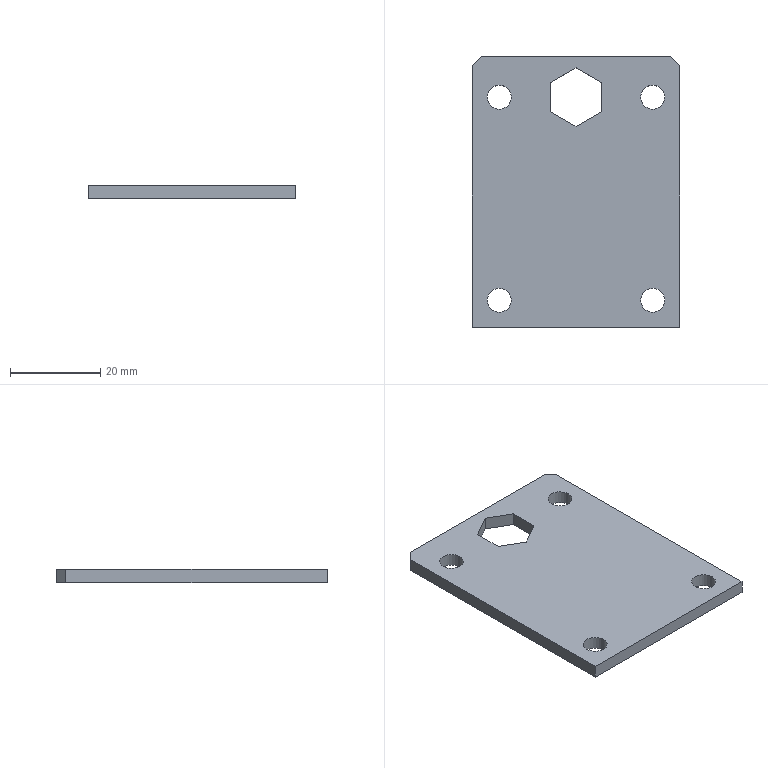Part | STEP file | Z-081D | 1 solid | 18 faces | box 46 x 60 x 2.9 mm | volume 7421 mm3 | plane 14 | cylinder 4 | commonest cylinder face diameters 5.3 x4
STEP:
#1=CARTESIAN_POINT('',(0.,0.,0.));
#2=DIRECTION('',(0.,0.,1.));
#3=DIRECTION('',(1.,0.,0.));
#4=AXIS2_PLACEMENT_3D('',#1,#2,#3);
#5=CARTESIAN_POINT('',(17.4,54.233,2.9));
#6=VERTEX_POINT('',#5);
#7=CARTESIAN_POINT('',(23.,57.466,2.9));
#8=VERTEX_POINT('',#7);
#9=CARTESIAN_POINT('',(14.253,52.416,2.9));
#10=DIRECTION('',(0.866,0.5,0.));
#11=VECTOR('',#10,1.);
#12=LINE('',#9,#11);
#13=CARTESIAN_POINT('',(17.4,54.233,2.9));
#14=DIRECTION('',(-0.5,0.866,0.));
#15=DIRECTION('',(0.866,0.5,0.));
#16=AXIS2_PLACEMENT_3D('',#13,#14,#15);
#17=PLANE('',#16);
#18=CARTESIAN_POINT('',(-3.633,0.));
#19=DIRECTION('',(1.,0.));
#20=VECTOR('',#19,1.);
#21=LINE('',#18,#20);
#22=(GEOMETRIC_REPRESENTATION_CONTEXT(2)PARAMETRIC_REPRESENTATION_CONTEXT()REPRESENTATION_CONTEXT('',''));
#23=DEFINITIONAL_REPRESENTATION('',(#21),#22);
#24=PCURVE('',#17,#23);
#25=CARTESIAN_POINT('',(23.,30.,2.9));
#26=DIRECTION('',(0.,0.,1.));
#27=DIRECTION('',(1.,0.,0.));
#28=AXIS2_PLACEMENT_3D('',#25,#26,#27);
#29=PLANE('',#28);
#30=CARTESIAN_POINT('',(-8.747,22.416));
#31=DIRECTION('',(0.866,0.5));
#32=VECTOR('',#31,1.);
#33=LINE('',#30,#32);
#34=(GEOMETRIC_REPRESENTATION_CONTEXT(2)PARAMETRIC_REPRESENTATION_CONTEXT()REPRESENTATION_CONTEXT('',''));
#35=DEFINITIONAL_REPRESENTATION('',(#33),#34);
#36=PCURVE('',#29,#35);
#37=SURFACE_CURVE('',#12,(#24,#36),.PCURVE_S1.);
#38=EDGE_CURVE('',#6,#8,#37,.T.);
#39=ORIENTED_EDGE('',*,*,#38,.F.);
#40=CARTESIAN_POINT('',(17.4,54.233,0.));
#41=VERTEX_POINT('',#40);
#42=CARTESIAN_POINT('',(17.4,54.233,2.9));
#43=DIRECTION('',(0.,0.,-1.));
#44=VECTOR('',#43,1.);
#45=LINE('',#42,#44);
#46=CARTESIAN_POINT('',(0.,0.));
#47=DIRECTION('',(0.,1.));
#48=VECTOR('',#47,1.);
#49=LINE('',#46,#48);
#50=(GEOMETRIC_REPRESENTATION_CONTEXT(2)PARAMETRIC_REPRESENTATION_CONTEXT()REPRESENTATION_CONTEXT('',''));
#51=DEFINITIONAL_REPRESENTATION('',(#49),#50);
#52=PCURVE('',#17,#51);
#53=CARTESIAN_POINT('',(17.4,47.767,2.9));
#54=DIRECTION('',(-1.,0.,0.));
#55=DIRECTION('',(0.,1.,0.));
#56=AXIS2_PLACEMENT_3D('',#53,#54,#55);
#57=PLANE('',#56);
#58=CARTESIAN_POINT('',(6.466,0.));
#59=DIRECTION('',(0.,1.));
#60=VECTOR('',#59,1.);
#61=LINE('',#58,#60);
#62=(GEOMETRIC_REPRESENTATION_CONTEXT(2)PARAMETRIC_REPRESENTATION_CONTEXT()REPRESENTATION_CONTEXT('',''));
#63=DEFINITIONAL_REPRESENTATION('',(#61),#62);
#64=PCURVE('',#57,#63);
#65=SURFACE_CURVE('',#45,(#52,#64),.PCURVE_S1.);
#66=EDGE_CURVE('',#6,#41,#65,.T.);
#67=ORIENTED_EDGE('',*,*,#66,.T.);
#68=CARTESIAN_POINT('',(23.,57.466,0.));
#69=VERTEX_POINT('',#68);
#70=CARTESIAN_POINT('',(14.253,52.416,0.));
#71=DIRECTION('',(-0.866,-0.5,0.));
#72=VECTOR('',#71,1.);
#73=LINE('',#70,#72);
#74=CARTESIAN_POINT('',(-3.633,2.9));
#75=DIRECTION('',(-1.,0.));
#76=VECTOR('',#75,1.);
#77=LINE('',#74,#76);
#78=(GEOMETRIC_REPRESENTATION_CONTEXT(2)PARAMETRIC_REPRESENTATION_CONTEXT()REPRESENTATION_CONTEXT('',''));
#79=DEFINITIONAL_REPRESENTATION('',(#77),#78);
#80=PCURVE('',#17,#79);
#81=CARTESIAN_POINT('',(23.,30.,0.));
#82=DIRECTION('',(0.,0.,1.));
#83=DIRECTION('',(1.,0.,0.));
#84=AXIS2_PLACEMENT_3D('',#81,#82,#83);
#85=PLANE('',#84);
#86=CARTESIAN_POINT('',(-8.747,22.416));
#87=DIRECTION('',(-0.866,-0.5));
#88=VECTOR('',#87,1.);
#89=LINE('',#86,#88);
#90=(GEOMETRIC_REPRESENTATION_CONTEXT(2)PARAMETRIC_REPRESENTATION_CONTEXT()REPRESENTATION_CONTEXT('',''));
#91=DEFINITIONAL_REPRESENTATION('',(#89),#90);
#92=PCURVE('',#85,#91);
#93=SURFACE_CURVE('',#73,(#80,#92),.PCURVE_S1.);
#94=EDGE_CURVE('',#69,#41,#93,.T.);
#95=ORIENTED_EDGE('',*,*,#94,.F.);
#96=CARTESIAN_POINT('',(23.,57.466,2.9));
#97=DIRECTION('',(0.,0.,-1.));
#98=VECTOR('',#97,1.);
#99=LINE('',#96,#98);
#100=CARTESIAN_POINT('',(6.466,0.));
#101=DIRECTION('',(0.,1.));
#102=VECTOR('',#101,1.);
#103=LINE('',#100,#102);
#104=(GEOMETRIC_REPRESENTATION_CONTEXT(2)PARAMETRIC_REPRESENTATION_CONTEXT()REPRESENTATION_CONTEXT('',''));
#105=DEFINITIONAL_REPRESENTATION('',(#103),#104);
#106=PCURVE('',#17,#105);
#107=CARTESIAN_POINT('',(23.,57.466,2.9));
#108=DIRECTION('',(0.5,0.866,0.));
#109=DIRECTION('',(0.866,-0.5,0.));
#110=AXIS2_PLACEMENT_3D('',#107,#108,#109);
#111=PLANE('',#110);
#112=CARTESIAN_POINT('',(0.,0.));
#113=DIRECTION('',(0.,1.));
#114=VECTOR('',#113,1.);
#115=LINE('',#112,#114);
#116=(GEOMETRIC_REPRESENTATION_CONTEXT(2)PARAMETRIC_REPRESENTATION_CONTEXT()REPRESENTATION_CONTEXT('',''));
#117=DEFINITIONAL_REPRESENTATION('',(#115),#116);
#118=PCURVE('',#111,#117);
#119=SURFACE_CURVE('',#99,(#106,#118),.PCURVE_S1.);
#120=EDGE_CURVE('',#8,#69,#119,.T.);
#121=ORIENTED_EDGE('',*,*,#120,.F.);
#122=EDGE_LOOP('',(#39,#67,#95,#121));
#123=FACE_BOUND('',#122,.T.);
#124=ADVANCED_FACE('',(#123),#17,.F.);
#125=CARTESIAN_POINT('',(17.4,47.767,2.9));
#126=VERTEX_POINT('',#125);
#127=CARTESIAN_POINT('',(17.4,38.883,2.9));
#128=DIRECTION('',(0.,1.,0.));
#129=VECTOR('',#128,1.);
#130=LINE('',#127,#129);
#131=CARTESIAN_POINT('',(-8.883,0.));
#132=DIRECTION('',(1.,0.));
#133=VECTOR('',#132,1.);
#134=LINE('',#131,#133);
#135=(GEOMETRIC_REPRESENTATION_CONTEXT(2)PARAMETRIC_REPRESENTATION_CONTEXT()REPRESENTATION_CONTEXT('',''));
#136=DEFINITIONAL_REPRESENTATION('',(#134),#135);
#137=PCURVE('',#57,#136);
#138=CARTESIAN_POINT('',(-5.6,8.883));
#139=DIRECTION('',(0.,1.));
#140=VECTOR('',#139,1.);
#141=LINE('',#138,#140);
#142=(GEOMETRIC_REPRESENTATION_CONTEXT(2)PARAMETRIC_REPRESENTATION_CONTEXT()REPRESENTATION_CONTEXT('',''));
#143=DEFINITIONAL_REPRESENTATION('',(#141),#142);
#144=PCURVE('',#29,#143);
#145=SURFACE_CURVE('',#130,(#137,#144),.PCURVE_S1.);
#146=EDGE_CURVE('',#126,#6,#145,.T.);
#147=ORIENTED_EDGE('',*,*,#146,.F.);
#148=CARTESIAN_POINT('',(17.4,47.767,0.));
#149=VERTEX_POINT('',#148);
#150=CARTESIAN_POINT('',(17.4,47.767,2.9));
#151=DIRECTION('',(0.,0.,-1.));
#152=VECTOR('',#151,1.);
#153=LINE('',#150,#152);
#154=CARTESIAN_POINT('',(0.,0.));
#155=DIRECTION('',(0.,1.));
#156=VECTOR('',#155,1.);
#157=LINE('',#154,#156);
#158=(GEOMETRIC_REPRESENTATION_CONTEXT(2)PARAMETRIC_REPRESENTATION_CONTEXT()REPRESENTATION_CONTEXT('',''));
#159=DEFINITIONAL_REPRESENTATION('',(#157),#158);
#160=PCURVE('',#57,#159);
#161=CARTESIAN_POINT('',(23.,44.534,2.9));
#162=DIRECTION('',(-0.5,-0.866,0.));
#163=DIRECTION('',(-0.866,0.5,0.));
#164=AXIS2_PLACEMENT_3D('',#161,#162,#163);
#165=PLANE('',#164);
#166=CARTESIAN_POINT('',(6.466,0.));
#167=DIRECTION('',(0.,1.));
#168=VECTOR('',#167,1.);
#169=LINE('',#166,#168);
#170=(GEOMETRIC_REPRESENTATION_CONTEXT(2)PARAMETRIC_REPRESENTATION_CONTEXT()REPRESENTATION_CONTEXT('',''));
#171=DEFINITIONAL_REPRESENTATION('',(#169),#170);
#172=PCURVE('',#165,#171);
#173=SURFACE_CURVE('',#153,(#160,#172),.PCURVE_S1.);
#174=EDGE_CURVE('',#126,#149,#173,.T.);
#175=ORIENTED_EDGE('',*,*,#174,.T.);
#176=CARTESIAN_POINT('',(17.4,38.883,0.));
#177=DIRECTION('',(0.,-1.,0.));
#178=VECTOR('',#177,1.);
#179=LINE('',#176,#178);
#180=CARTESIAN_POINT('',(-8.883,2.9));
#181=DIRECTION('',(-1.,0.));
#182=VECTOR('',#181,1.);
#183=LINE('',#180,#182);
#184=(GEOMETRIC_REPRESENTATION_CONTEXT(2)PARAMETRIC_REPRESENTATION_CONTEXT()REPRESENTATION_CONTEXT('',''));
#185=DEFINITIONAL_REPRESENTATION('',(#183),#184);
#186=PCURVE('',#57,#185);
#187=CARTESIAN_POINT('',(-5.6,8.883));
#188=DIRECTION('',(0.,-1.));
#189=VECTOR('',#188,1.);
#190=LINE('',#187,#189);
#191=(GEOMETRIC_REPRESENTATION_CONTEXT(2)PARAMETRIC_REPRESENTATION_CONTEXT()REPRESENTATION_CONTEXT('',''));
#192=DEFINITIONAL_REPRESENTATION('',(#190),#191);
#193=PCURVE('',#85,#192);
#194=SURFACE_CURVE('',#179,(#186,#193),.PCURVE_S1.);
#195=EDGE_CURVE('',#41,#149,#194,.T.);
#196=ORIENTED_EDGE('',*,*,#195,.F.);
#197=ORIENTED_EDGE('',*,*,#66,.F.);
#198=EDGE_LOOP('',(#147,#175,#196,#197));
#199=FACE_BOUND('',#198,.T.);
#200=ADVANCED_FACE('',(#199),#57,.F.);
#201=CARTESIAN_POINT('',(23.,44.534,2.9));
#202=VERTEX_POINT('',#201);
#203=CARTESIAN_POINT('',(26.147,42.717,2.9));
#204=DIRECTION('',(-0.866,0.5,0.));
#205=VECTOR('',#204,1.);
#206=LINE('',#203,#205);
#207=CARTESIAN_POINT('',(-3.633,0.));
#208=DIRECTION('',(1.,0.));
#209=VECTOR('',#208,1.);
#210=LINE('',#207,#209);
#211=(GEOMETRIC_REPRESENTATION_CONTEXT(2)PARAMETRIC_REPRESENTATION_CONTEXT()REPRESENTATION_CONTEXT('',''));
#212=DEFINITIONAL_REPRESENTATION('',(#210),#211);
#213=PCURVE('',#165,#212);
#214=CARTESIAN_POINT('',(3.147,12.717));
#215=DIRECTION('',(-0.866,0.5));
#216=VECTOR('',#215,1.);
#217=LINE('',#214,#216);
#218=(GEOMETRIC_REPRESENTATION_CONTEXT(2)PARAMETRIC_REPRESENTATION_CONTEXT()REPRESENTATION_CONTEXT('',''));
#219=DEFINITIONAL_REPRESENTATION('',(#217),#218);
#220=PCURVE('',#29,#219);
#221=SURFACE_CURVE('',#206,(#213,#220),.PCURVE_S1.);
#222=EDGE_CURVE('',#202,#126,#221,.T.);
#223=ORIENTED_EDGE('',*,*,#222,.F.);
#224=CARTESIAN_POINT('',(23.,44.534,0.));
#225=VERTEX_POINT('',#224);
#226=CARTESIAN_POINT('',(23.,44.534,2.9));
#227=DIRECTION('',(0.,0.,-1.));
#228=VECTOR('',#227,1.);
#229=LINE('',#226,#228);
#230=CARTESIAN_POINT('',(0.,0.));
#231=DIRECTION('',(0.,1.));
#232=VECTOR('',#231,1.);
#233=LINE('',#230,#232);
#234=(GEOMETRIC_REPRESENTATION_CONTEXT(2)PARAMETRIC_REPRESENTATION_CONTEXT()REPRESENTATION_CONTEXT('',''));
#235=DEFINITIONAL_REPRESENTATION('',(#233),#234);
#236=PCURVE('',#165,#235);
#237=CARTESIAN_POINT('',(28.6,47.767,2.9));
#238=DIRECTION('',(0.5,-0.866,0.));
#239=DIRECTION('',(-0.866,-0.5,0.));
#240=AXIS2_PLACEMENT_3D('',#237,#238,#239);
#241=PLANE('',#240);
#242=CARTESIAN_POINT('',(6.466,0.));
#243=DIRECTION('',(0.,1.));
#244=VECTOR('',#243,1.);
#245=LINE('',#242,#244);
#246=(GEOMETRIC_REPRESENTATION_CONTEXT(2)PARAMETRIC_REPRESENTATION_CONTEXT()REPRESENTATION_CONTEXT('',''));
#247=DEFINITIONAL_REPRESENTATION('',(#245),#246);
#248=PCURVE('',#241,#247);
#249=SURFACE_CURVE('',#229,(#236,#248),.PCURVE_S1.);
#250=EDGE_CURVE('',#202,#225,#249,.T.);
#251=ORIENTED_EDGE('',*,*,#250,.T.);
#252=CARTESIAN_POINT('',(26.147,42.717,0.));
#253=DIRECTION('',(0.866,-0.5,0.));
#254=VECTOR('',#253,1.);
#255=LINE('',#252,#254);
#256=CARTESIAN_POINT('',(-3.633,2.9));
#257=DIRECTION('',(-1.,0.));
#258=VECTOR('',#257,1.);
#259=LINE('',#256,#258);
#260=(GEOMETRIC_REPRESENTATION_CONTEXT(2)PARAMETRIC_REPRESENTATION_CONTEXT()REPRESENTATION_CONTEXT('',''));
#261=DEFINITIONAL_REPRESENTATION('',(#259),#260);
#262=PCURVE('',#165,#261);
#263=CARTESIAN_POINT('',(3.147,12.717));
#264=DIRECTION('',(0.866,-0.5));
#265=VECTOR('',#264,1.);
#266=LINE('',#263,#265);
#267=(GEOMETRIC_REPRESENTATION_CONTEXT(2)PARAMETRIC_REPRESENTATION_CONTEXT()REPRESENTATION_CONTEXT('',''));
#268=DEFINITIONAL_REPRESENTATION('',(#266),#267);
#269=PCURVE('',#85,#268);
#270=SURFACE_CURVE('',#255,(#262,#269),.PCURVE_S1.);
#271=EDGE_CURVE('',#149,#225,#270,.T.);
#272=ORIENTED_EDGE('',*,*,#271,.F.);
#273=ORIENTED_EDGE('',*,*,#174,.F.);
#274=EDGE_LOOP('',(#223,#251,#272,#273));
#275=FACE_BOUND('',#274,.T.);
#276=ADVANCED_FACE('',(#275),#165,.F.);
#277=CARTESIAN_POINT('',(28.6,47.767,2.9));
#278=VERTEX_POINT('',#277);
#279=CARTESIAN_POINT('',(22.653,44.334,2.9));
#280=DIRECTION('',(-0.866,-0.5,0.));
#281=VECTOR('',#280,1.);
#282=LINE('',#279,#281);
#283=CARTESIAN_POINT('',(6.867,0.));
#284=DIRECTION('',(1.,0.));
#285=VECTOR('',#284,1.);
#286=LINE('',#283,#285);
#287=(GEOMETRIC_REPRESENTATION_CONTEXT(2)PARAMETRIC_REPRESENTATION_CONTEXT()REPRESENTATION_CONTEXT('',''));
#288=DEFINITIONAL_REPRESENTATION('',(#286),#287);
#289=PCURVE('',#241,#288);
#290=CARTESIAN_POINT('',(-0.3466,14.334));
#291=DIRECTION('',(-0.866,-0.5));
#292=VECTOR('',#291,1.);
#293=LINE('',#290,#292);
#294=(GEOMETRIC_REPRESENTATION_CONTEXT(2)PARAMETRIC_REPRESENTATION_CONTEXT()REPRESENTATION_CONTEXT('',''));
#295=DEFINITIONAL_REPRESENTATION('',(#293),#294);
#296=PCURVE('',#29,#295);
#297=SURFACE_CURVE('',#282,(#289,#296),.PCURVE_S1.);
#298=EDGE_CURVE('',#278,#202,#297,.T.);
#299=ORIENTED_EDGE('',*,*,#298,.F.);
#300=CARTESIAN_POINT('',(28.6,47.767,0.));
#301=VERTEX_POINT('',#300);
#302=CARTESIAN_POINT('',(28.6,47.767,2.9));
#303=DIRECTION('',(0.,0.,-1.));
#304=VECTOR('',#303,1.);
#305=LINE('',#302,#304);
#306=CARTESIAN_POINT('',(0.,0.));
#307=DIRECTION('',(0.,1.));
#308=VECTOR('',#307,1.);
#309=LINE('',#306,#308);
#310=(GEOMETRIC_REPRESENTATION_CONTEXT(2)PARAMETRIC_REPRESENTATION_CONTEXT()REPRESENTATION_CONTEXT('',''));
#311=DEFINITIONAL_REPRESENTATION('',(#309),#310);
#312=PCURVE('',#241,#311);
#313=CARTESIAN_POINT('',(28.6,54.233,2.9));
#314=DIRECTION('',(1.,0.,0.));
#315=DIRECTION('',(0.,-1.,0.));
#316=AXIS2_PLACEMENT_3D('',#313,#314,#315);
#317=PLANE('',#316);
#318=CARTESIAN_POINT('',(6.466,0.));
#319=DIRECTION('',(0.,1.));
#320=VECTOR('',#319,1.);
#321=LINE('',#318,#320);
#322=(GEOMETRIC_REPRESENTATION_CONTEXT(2)PARAMETRIC_REPRESENTATION_CONTEXT()REPRESENTATION_CONTEXT('',''));
#323=DEFINITIONAL_REPRESENTATION('',(#321),#322);
#324=PCURVE('',#317,#323);
#325=SURFACE_CURVE('',#305,(#312,#324),.PCURVE_S1.);
#326=EDGE_CURVE('',#278,#301,#325,.T.);
#327=ORIENTED_EDGE('',*,*,#326,.T.);
#328=CARTESIAN_POINT('',(22.653,44.334,0.));
#329=DIRECTION('',(0.866,0.5,0.));
#330=VECTOR('',#329,1.);
#331=LINE('',#328,#330);
#332=CARTESIAN_POINT('',(6.867,2.9));
#333=DIRECTION('',(-1.,0.));
#334=VECTOR('',#333,1.);
#335=LINE('',#332,#334);
#336=(GEOMETRIC_REPRESENTATION_CONTEXT(2)PARAMETRIC_REPRESENTATION_CONTEXT()REPRESENTATION_CONTEXT('',''));
#337=DEFINITIONAL_REPRESENTATION('',(#335),#336);
#338=PCURVE('',#241,#337);
#339=CARTESIAN_POINT('',(-0.3466,14.334));
#340=DIRECTION('',(0.866,0.5));
#341=VECTOR('',#340,1.);
#342=LINE('',#339,#341);
#343=(GEOMETRIC_REPRESENTATION_CONTEXT(2)PARAMETRIC_REPRESENTATION_CONTEXT()REPRESENTATION_CONTEXT('',''));
#344=DEFINITIONAL_REPRESENTATION('',(#342),#343);
#345=PCURVE('',#85,#344);
#346=SURFACE_CURVE('',#331,(#338,#345),.PCURVE_S1.);
#347=EDGE_CURVE('',#225,#301,#346,.T.);
#348=ORIENTED_EDGE('',*,*,#347,.F.);
#349=ORIENTED_EDGE('',*,*,#250,.F.);
#350=EDGE_LOOP('',(#299,#327,#348,#349));
#351=FACE_BOUND('',#350,.T.);
#352=ADVANCED_FACE('',(#351),#241,.F.);
#353=CARTESIAN_POINT('',(28.6,54.233,2.9));
#354=VERTEX_POINT('',#353);
#355=CARTESIAN_POINT('',(28.6,42.117,2.9));
#356=DIRECTION('',(0.,-1.,0.));
#357=VECTOR('',#356,1.);
#358=LINE('',#355,#357);
#359=CARTESIAN_POINT('',(12.117,0.));
#360=DIRECTION('',(1.,0.));
#361=VECTOR('',#360,1.);
#362=LINE('',#359,#361);
#363=(GEOMETRIC_REPRESENTATION_CONTEXT(2)PARAMETRIC_REPRESENTATION_CONTEXT()REPRESENTATION_CONTEXT('',''));
#364=DEFINITIONAL_REPRESENTATION('',(#362),#363);
#365=PCURVE('',#317,#364);
#366=CARTESIAN_POINT('',(5.6,12.117));
#367=DIRECTION('',(0.,-1.));
#368=VECTOR('',#367,1.);
#369=LINE('',#366,#368);
#370=(GEOMETRIC_REPRESENTATION_CONTEXT(2)PARAMETRIC_REPRESENTATION_CONTEXT()REPRESENTATION_CONTEXT('',''));
#371=DEFINITIONAL_REPRESENTATION('',(#369),#370);
#372=PCURVE('',#29,#371);
#373=SURFACE_CURVE('',#358,(#365,#372),.PCURVE_S1.);
#374=EDGE_CURVE('',#354,#278,#373,.T.);
#375=ORIENTED_EDGE('',*,*,#374,.F.);
#376=CARTESIAN_POINT('',(28.6,54.233,0.));
#377=VERTEX_POINT('',#376);
#378=CARTESIAN_POINT('',(28.6,54.233,2.9));
#379=DIRECTION('',(0.,0.,-1.));
#380=VECTOR('',#379,1.);
#381=LINE('',#378,#380);
#382=CARTESIAN_POINT('',(0.,0.));
#383=DIRECTION('',(0.,1.));
#384=VECTOR('',#383,1.);
#385=LINE('',#382,#384);
#386=(GEOMETRIC_REPRESENTATION_CONTEXT(2)PARAMETRIC_REPRESENTATION_CONTEXT()REPRESENTATION_CONTEXT('',''));
#387=DEFINITIONAL_REPRESENTATION('',(#385),#386);
#388=PCURVE('',#317,#387);
#389=CARTESIAN_POINT('',(6.466,0.));
#390=DIRECTION('',(0.,1.));
#391=VECTOR('',#390,1.);
#392=LINE('',#389,#391);
#393=(GEOMETRIC_REPRESENTATION_CONTEXT(2)PARAMETRIC_REPRESENTATION_CONTEXT()REPRESENTATION_CONTEXT('',''));
#394=DEFINITIONAL_REPRESENTATION('',(#392),#393);
#395=PCURVE('',#111,#394);
#396=SURFACE_CURVE('',#381,(#388,#395),.PCURVE_S1.);
#397=EDGE_CURVE('',#354,#377,#396,.T.);
#398=ORIENTED_EDGE('',*,*,#397,.T.);
#399=CARTESIAN_POINT('',(28.6,42.117,0.));
#400=DIRECTION('',(0.,1.,0.));
#401=VECTOR('',#400,1.);
#402=LINE('',#399,#401);
#403=CARTESIAN_POINT('',(12.117,2.9));
#404=DIRECTION('',(-1.,0.));
#405=VECTOR('',#404,1.);
#406=LINE('',#403,#405);
#407=(GEOMETRIC_REPRESENTATION_CONTEXT(2)PARAMETRIC_REPRESENTATION_CONTEXT()REPRESENTATION_CONTEXT('',''));
#408=DEFINITIONAL_REPRESENTATION('',(#406),#407);
#409=PCURVE('',#317,#408);
#410=CARTESIAN_POINT('',(5.6,12.117));
#411=DIRECTION('',(0.,1.));
#412=VECTOR('',#411,1.);
#413=LINE('',#410,#412);
#414=(GEOMETRIC_REPRESENTATION_CONTEXT(2)PARAMETRIC_REPRESENTATION_CONTEXT()REPRESENTATION_CONTEXT('',''));
#415=DEFINITIONAL_REPRESENTATION('',(#413),#414);
#416=PCURVE('',#85,#415);
#417=SURFACE_CURVE('',#402,(#409,#416),.PCURVE_S1.);
#418=EDGE_CURVE('',#301,#377,#417,.T.);
#419=ORIENTED_EDGE('',*,*,#418,.F.);
#420=ORIENTED_EDGE('',*,*,#326,.F.);
#421=EDGE_LOOP('',(#375,#398,#419,#420));
#422=FACE_BOUND('',#421,.T.);
#423=ADVANCED_FACE('',(#422),#317,.F.);
#424=CARTESIAN_POINT('',(28.947,54.033,2.9));
#425=DIRECTION('',(0.866,-0.5,0.));
#426=VECTOR('',#425,1.);
#427=LINE('',#424,#426);
#428=CARTESIAN_POINT('',(6.867,0.));
#429=DIRECTION('',(1.,0.));
#430=VECTOR('',#429,1.);
#431=LINE('',#428,#430);
#432=(GEOMETRIC_REPRESENTATION_CONTEXT(2)PARAMETRIC_REPRESENTATION_CONTEXT()REPRESENTATION_CONTEXT('',''));
#433=DEFINITIONAL_REPRESENTATION('',(#431),#432);
#434=PCURVE('',#111,#433);
#435=CARTESIAN_POINT('',(5.947,24.033));
#436=DIRECTION('',(0.866,-0.5));
#437=VECTOR('',#436,1.);
#438=LINE('',#435,#437);
#439=(GEOMETRIC_REPRESENTATION_CONTEXT(2)PARAMETRIC_REPRESENTATION_CONTEXT()REPRESENTATION_CONTEXT('',''));
#440=DEFINITIONAL_REPRESENTATION('',(#438),#439);
#441=PCURVE('',#29,#440);
#442=SURFACE_CURVE('',#427,(#434,#441),.PCURVE_S1.);
#443=EDGE_CURVE('',#8,#354,#442,.T.);
#444=ORIENTED_EDGE('',*,*,#443,.F.);
#445=ORIENTED_EDGE('',*,*,#120,.T.);
#446=CARTESIAN_POINT('',(28.947,54.033,0.));
#447=DIRECTION('',(-0.866,0.5,0.));
#448=VECTOR('',#447,1.);
#449=LINE('',#446,#448);
#450=CARTESIAN_POINT('',(6.867,2.9));
#451=DIRECTION('',(-1.,0.));
#452=VECTOR('',#451,1.);
#453=LINE('',#450,#452);
#454=(GEOMETRIC_REPRESENTATION_CONTEXT(2)PARAMETRIC_REPRESENTATION_CONTEXT()REPRESENTATION_CONTEXT('',''));
#455=DEFINITIONAL_REPRESENTATION('',(#453),#454);
#456=PCURVE('',#111,#455);
#457=CARTESIAN_POINT('',(5.947,24.033));
#458=DIRECTION('',(-0.866,0.5));
#459=VECTOR('',#458,1.);
#460=LINE('',#457,#459);
#461=(GEOMETRIC_REPRESENTATION_CONTEXT(2)PARAMETRIC_REPRESENTATION_CONTEXT()REPRESENTATION_CONTEXT('',''));
#462=DEFINITIONAL_REPRESENTATION('',(#460),#461);
#463=PCURVE('',#85,#462);
#464=SURFACE_CURVE('',#449,(#456,#463),.PCURVE_S1.);
#465=EDGE_CURVE('',#377,#69,#464,.T.);
#466=ORIENTED_EDGE('',*,*,#465,.F.);
#467=ORIENTED_EDGE('',*,*,#397,.F.);
#468=EDGE_LOOP('',(#444,#445,#466,#467));
#469=FACE_BOUND('',#468,.T.);
#470=ADVANCED_FACE('',(#469),#111,.F.);
#471=CARTESIAN_POINT('',(0.,58.,2.9));
#472=VERTEX_POINT('',#471);
#473=CARTESIAN_POINT('',(2.,60.,2.9));
#474=VERTEX_POINT('',#473);
#475=CARTESIAN_POINT('',(-0.75,57.25,2.9));
#476=DIRECTION('',(0.7071,0.7071,0.));
#477=VECTOR('',#476,1.);
#478=LINE('',#475,#477);
#479=CARTESIAN_POINT('',(1.,59.,0.));
#480=DIRECTION('',(-0.7071,0.7071,0.));
#481=DIRECTION('',(0.,0.,1.));
#482=AXIS2_PLACEMENT_3D('',#479,#480,#481);
#483=PLANE('',#482);
#484=CARTESIAN_POINT('',(2.9,-2.475));
#485=DIRECTION('',(0.,1.));
#486=VECTOR('',#485,1.);
#487=LINE('',#484,#486);
#488=(GEOMETRIC_REPRESENTATION_CONTEXT(2)PARAMETRIC_REPRESENTATION_CONTEXT()REPRESENTATION_CONTEXT('',''));
#489=DEFINITIONAL_REPRESENTATION('',(#487),#488);
#490=PCURVE('',#483,#489);
#491=CARTESIAN_POINT('',(-23.75,27.25));
#492=DIRECTION('',(0.7071,0.7071));
#493=VECTOR('',#492,1.);
#494=LINE('',#491,#493);
#495=(GEOMETRIC_REPRESENTATION_CONTEXT(2)PARAMETRIC_REPRESENTATION_CONTEXT()REPRESENTATION_CONTEXT('',''));
#496=DEFINITIONAL_REPRESENTATION('',(#494),#495);
#497=PCURVE('',#29,#496);
#498=SURFACE_CURVE('',#478,(#490,#497),.PCURVE_S1.);
#499=EDGE_CURVE('',#472,#474,#498,.T.);
#500=ORIENTED_EDGE('',*,*,#499,.T.);
#501=CARTESIAN_POINT('',(2.,60.,0.));
#502=VERTEX_POINT('',#501);
#503=CARTESIAN_POINT('',(2.,60.,0.));
#504=DIRECTION('',(0.,0.,-1.));
#505=VECTOR('',#504,1.);
#506=LINE('',#503,#505);
#507=CARTESIAN_POINT('',(0.,1.414));
#508=DIRECTION('',(-1.,0.));
#509=VECTOR('',#508,1.);
#510=LINE('',#507,#509);
#511=(GEOMETRIC_REPRESENTATION_CONTEXT(2)PARAMETRIC_REPRESENTATION_CONTEXT()REPRESENTATION_CONTEXT('',''));
#512=DEFINITIONAL_REPRESENTATION('',(#510),#511);
#513=PCURVE('',#483,#512);
#514=CARTESIAN_POINT('',(0.,60.,0.));
#515=DIRECTION('',(0.,1.,0.));
#516=DIRECTION('',(0.,0.,1.));
#517=AXIS2_PLACEMENT_3D('',#514,#515,#516);
#518=PLANE('',#517);
#519=CARTESIAN_POINT('',(0.,2.));
#520=DIRECTION('',(-1.,0.));
#521=VECTOR('',#520,1.);
#522=LINE('',#519,#521);
#523=(GEOMETRIC_REPRESENTATION_CONTEXT(2)PARAMETRIC_REPRESENTATION_CONTEXT()REPRESENTATION_CONTEXT('',''));
#524=DEFINITIONAL_REPRESENTATION('',(#522),#523);
#525=PCURVE('',#518,#524);
#526=SURFACE_CURVE('',#506,(#513,#525),.PCURVE_S1.);
#527=EDGE_CURVE('',#474,#502,#526,.T.);
#528=ORIENTED_EDGE('',*,*,#527,.T.);
#529=CARTESIAN_POINT('',(0.,58.,0.));
#530=VERTEX_POINT('',#529);
#531=CARTESIAN_POINT('',(-0.75,57.25,0.));
#532=DIRECTION('',(-0.7071,-0.7071,0.));
#533=VECTOR('',#532,1.);
#534=LINE('',#531,#533);
#535=CARTESIAN_POINT('',(0.,-2.475));
#536=DIRECTION('',(0.,-1.));
#537=VECTOR('',#536,1.);
#538=LINE('',#535,#537);
#539=(GEOMETRIC_REPRESENTATION_CONTEXT(2)PARAMETRIC_REPRESENTATION_CONTEXT()REPRESENTATION_CONTEXT('',''));
#540=DEFINITIONAL_REPRESENTATION('',(#538),#539);
#541=PCURVE('',#483,#540);
#542=CARTESIAN_POINT('',(-23.75,27.25));
#543=DIRECTION('',(-0.7071,-0.7071));
#544=VECTOR('',#543,1.);
#545=LINE('',#542,#544);
#546=(GEOMETRIC_REPRESENTATION_CONTEXT(2)PARAMETRIC_REPRESENTATION_CONTEXT()REPRESENTATION_CONTEXT('',''));
#547=DEFINITIONAL_REPRESENTATION('',(#545),#546);
#548=PCURVE('',#85,#547);
#549=SURFACE_CURVE('',#534,(#541,#548),.PCURVE_S1.);
#550=EDGE_CURVE('',#502,#530,#549,.T.);
#551=ORIENTED_EDGE('',*,*,#550,.T.);
#552=CARTESIAN_POINT('',(0.,58.,0.));
#553=DIRECTION('',(0.,0.,1.));
#554=VECTOR('',#553,1.);
#555=LINE('',#552,#554);
#556=CARTESIAN_POINT('',(0.,-1.414));
#557=DIRECTION('',(1.,0.));
#558=VECTOR('',#557,1.);
#559=LINE('',#556,#558);
#560=(GEOMETRIC_REPRESENTATION_CONTEXT(2)PARAMETRIC_REPRESENTATION_CONTEXT()REPRESENTATION_CONTEXT('',''));
#561=DEFINITIONAL_REPRESENTATION('',(#559),#560);
#562=PCURVE('',#483,#561);
#563=CARTESIAN_POINT('',(0.,0.,0.));
#564=DIRECTION('',(-1.,0.,0.));
#565=DIRECTION('',(0.,0.,1.));
#566=AXIS2_PLACEMENT_3D('',#563,#564,#565);
#567=PLANE('',#566);
#568=CARTESIAN_POINT('',(0.,58.));
#569=DIRECTION('',(1.,0.));
#570=VECTOR('',#569,1.);
#571=LINE('',#568,#570);
#572=(GEOMETRIC_REPRESENTATION_CONTEXT(2)PARAMETRIC_REPRESENTATION_CONTEXT()REPRESENTATION_CONTEXT('',''));
#573=DEFINITIONAL_REPRESENTATION('',(#571),#572);
#574=PCURVE('',#567,#573);
#575=SURFACE_CURVE('',#555,(#562,#574),.PCURVE_S1.);
#576=EDGE_CURVE('',#530,#472,#575,.T.);
#577=ORIENTED_EDGE('',*,*,#576,.T.);
#578=EDGE_LOOP('',(#500,#528,#551,#577));
#579=FACE_BOUND('',#578,.T.);
#580=ADVANCED_FACE('',(#579),#483,.T.);
#581=ORIENTED_EDGE('',*,*,#576,.F.);
#582=CARTESIAN_POINT('',(0.,0.,0.));
#583=VERTEX_POINT('',#582);
#584=CARTESIAN_POINT('',(0.,60.,0.));
#585=DIRECTION('',(0.,-1.,0.));
#586=VECTOR('',#585,1.);
#587=LINE('',#584,#586);
#588=CARTESIAN_POINT('',(0.,60.));
#589=DIRECTION('',(0.,-1.));
#590=VECTOR('',#589,1.);
#591=LINE('',#588,#590);
#592=(GEOMETRIC_REPRESENTATION_CONTEXT(2)PARAMETRIC_REPRESENTATION_CONTEXT()REPRESENTATION_CONTEXT('',''));
#593=DEFINITIONAL_REPRESENTATION('',(#591),#592);
#594=PCURVE('',#567,#593);
#595=CARTESIAN_POINT('',(-23.,30.));
#596=DIRECTION('',(0.,-1.));
#597=VECTOR('',#596,1.);
#598=LINE('',#595,#597);
#599=(GEOMETRIC_REPRESENTATION_CONTEXT(2)PARAMETRIC_REPRESENTATION_CONTEXT()REPRESENTATION_CONTEXT('',''));
#600=DEFINITIONAL_REPRESENTATION('',(#598),#599);
#601=PCURVE('',#85,#600);
#602=SURFACE_CURVE('',#587,(#594,#601),.PCURVE_S1.);
#603=EDGE_CURVE('',#530,#583,#602,.T.);
#604=ORIENTED_EDGE('',*,*,#603,.T.);
#605=CARTESIAN_POINT('',(0.,0.,2.9));
#606=VERTEX_POINT('',#605);
#607=CARTESIAN_POINT('',(0.,0.,0.));
#608=DIRECTION('',(0.,0.,1.));
#609=VECTOR('',#608,1.);
#610=LINE('',#607,#609);
#611=CARTESIAN_POINT('',(0.,0.));
#612=DIRECTION('',(1.,0.));
#613=VECTOR('',#612,1.);
#614=LINE('',#611,#613);
#615=(GEOMETRIC_REPRESENTATION_CONTEXT(2)PARAMETRIC_REPRESENTATION_CONTEXT()REPRESENTATION_CONTEXT('',''));
#616=DEFINITIONAL_REPRESENTATION('',(#614),#615);
#617=PCURVE('',#567,#616);
#618=CARTESIAN_POINT('',(46.,0.,0.));
#619=DIRECTION('',(0.,-1.,0.));
#620=DIRECTION('',(0.,0.,-1.));
#621=AXIS2_PLACEMENT_3D('',#618,#619,#620);
#622=PLANE('',#621);
#623=CARTESIAN_POINT('',(0.,-46.));
#624=DIRECTION('',(-1.,0.));
#625=VECTOR('',#624,1.);
#626=LINE('',#623,#625);
#627=(GEOMETRIC_REPRESENTATION_CONTEXT(2)PARAMETRIC_REPRESENTATION_CONTEXT()REPRESENTATION_CONTEXT('',''));
#628=DEFINITIONAL_REPRESENTATION('',(#626),#627);
#629=PCURVE('',#622,#628);
#630=SURFACE_CURVE('',#610,(#617,#629),.PCURVE_S1.);
#631=EDGE_CURVE('',#583,#606,#630,.T.);
#632=ORIENTED_EDGE('',*,*,#631,.T.);
#633=CARTESIAN_POINT('',(0.,60.,2.9));
#634=DIRECTION('',(0.,1.,0.));
#635=VECTOR('',#634,1.);
#636=LINE('',#633,#635);
#637=CARTESIAN_POINT('',(2.9,60.));
#638=DIRECTION('',(0.,1.));
#639=VECTOR('',#638,1.);
#640=LINE('',#637,#639);
#641=(GEOMETRIC_REPRESENTATION_CONTEXT(2)PARAMETRIC_REPRESENTATION_CONTEXT()REPRESENTATION_CONTEXT('',''));
#642=DEFINITIONAL_REPRESENTATION('',(#640),#641);
#643=PCURVE('',#567,#642);
#644=CARTESIAN_POINT('',(-23.,30.));
#645=DIRECTION('',(0.,1.));
#646=VECTOR('',#645,1.);
#647=LINE('',#644,#646);
#648=(GEOMETRIC_REPRESENTATION_CONTEXT(2)PARAMETRIC_REPRESENTATION_CONTEXT()REPRESENTATION_CONTEXT('',''));
#649=DEFINITIONAL_REPRESENTATION('',(#647),#648);
#650=PCURVE('',#29,#649);
#651=SURFACE_CURVE('',#636,(#643,#650),.PCURVE_S1.);
#652=EDGE_CURVE('',#606,#472,#651,.T.);
#653=ORIENTED_EDGE('',*,*,#652,.T.);
#654=EDGE_LOOP('',(#581,#604,#632,#653));
#655=FACE_BOUND('',#654,.T.);
#656=ADVANCED_FACE('',(#655),#567,.T.);
#657=ORIENTED_EDGE('',*,*,#550,.F.);
#658=CARTESIAN_POINT('',(44.,60.,0.));
#659=VERTEX_POINT('',#658);
#660=CARTESIAN_POINT('',(46.,60.,0.));
#661=DIRECTION('',(-1.,0.,0.));
#662=VECTOR('',#661,1.);
#663=LINE('',#660,#662);
#664=CARTESIAN_POINT('',(23.,30.));
#665=DIRECTION('',(-1.,0.));
#666=VECTOR('',#665,1.);
#667=LINE('',#664,#666);
#668=(GEOMETRIC_REPRESENTATION_CONTEXT(2)PARAMETRIC_REPRESENTATION_CONTEXT()REPRESENTATION_CONTEXT('',''));
#669=DEFINITIONAL_REPRESENTATION('',(#667),#668);
#670=PCURVE('',#85,#669);
#671=CARTESIAN_POINT('',(0.,46.));
#672=DIRECTION('',(0.,-1.));
#673=VECTOR('',#672,1.);
#674=LINE('',#671,#673);
#675=(GEOMETRIC_REPRESENTATION_CONTEXT(2)PARAMETRIC_REPRESENTATION_CONTEXT()REPRESENTATION_CONTEXT('',''));
#676=DEFINITIONAL_REPRESENTATION('',(#674),#675);
#677=PCURVE('',#518,#676);
#678=SURFACE_CURVE('',#663,(#670,#677),.PCURVE_S1.);
#679=EDGE_CURVE('',#659,#502,#678,.T.);
#680=ORIENTED_EDGE('',*,*,#679,.F.);
#681=CARTESIAN_POINT('',(46.,58.,0.));
#682=VERTEX_POINT('',#681);
#683=CARTESIAN_POINT('',(46.75,57.25,0.));
#684=DIRECTION('',(-0.7071,0.7071,0.));
#685=VECTOR('',#684,1.);
#686=LINE('',#683,#685);
#687=CARTESIAN_POINT('',(23.75,27.25));
#688=DIRECTION('',(-0.7071,0.7071));
#689=VECTOR('',#688,1.);
#690=LINE('',#687,#689);
#691=(GEOMETRIC_REPRESENTATION_CONTEXT(2)PARAMETRIC_REPRESENTATION_CONTEXT()REPRESENTATION_CONTEXT('',''));
#692=DEFINITIONAL_REPRESENTATION('',(#690),#691);
#693=PCURVE('',#85,#692);
#694=CARTESIAN_POINT('',(45.,59.,0.));
#695=DIRECTION('',(0.7071,0.7071,0.));
#696=DIRECTION('',(0.,0.,-1.));
#697=AXIS2_PLACEMENT_3D('',#694,#695,#696);
#698=PLANE('',#697);
#699=CARTESIAN_POINT('',(0.,-2.475));
#700=DIRECTION('',(0.,1.));
#701=VECTOR('',#700,1.);
#702=LINE('',#699,#701);
#703=(GEOMETRIC_REPRESENTATION_CONTEXT(2)PARAMETRIC_REPRESENTATION_CONTEXT()REPRESENTATION_CONTEXT('',''));
#704=DEFINITIONAL_REPRESENTATION('',(#702),#703);
#705=PCURVE('',#698,#704);
#706=SURFACE_CURVE('',#686,(#693,#705),.PCURVE_S1.);
#707=EDGE_CURVE('',#682,#659,#706,.T.);
#708=ORIENTED_EDGE('',*,*,#707,.F.);
#709=CARTESIAN_POINT('',(46.,0.,0.));
#710=VERTEX_POINT('',#709);
#711=CARTESIAN_POINT('',(46.,0.,0.));
#712=DIRECTION('',(0.,1.,0.));
#713=VECTOR('',#712,1.);
#714=LINE('',#711,#713);
#715=CARTESIAN_POINT('',(23.,-30.));
#716=DIRECTION('',(0.,1.));
#717=VECTOR('',#716,1.);
#718=LINE('',#715,#717);
#719=(GEOMETRIC_REPRESENTATION_CONTEXT(2)PARAMETRIC_REPRESENTATION_CONTEXT()REPRESENTATION_CONTEXT('',''));
#720=DEFINITIONAL_REPRESENTATION('',(#718),#719);
#721=PCURVE('',#85,#720);
#722=CARTESIAN_POINT('',(46.,60.,0.));
#723=DIRECTION('',(1.,0.,0.));
#724=DIRECTION('',(0.,0.,-1.));
#725=AXIS2_PLACEMENT_3D('',#722,#723,#724);
#726=PLANE('',#725);
#727=CARTESIAN_POINT('',(0.,-60.));
#728=DIRECTION('',(0.,1.));
#729=VECTOR('',#728,1.);
#730=LINE('',#727,#729);
#731=(GEOMETRIC_REPRESENTATION_CONTEXT(2)PARAMETRIC_REPRESENTATION_CONTEXT()REPRESENTATION_CONTEXT('',''));
#732=DEFINITIONAL_REPRESENTATION('',(#730),#731);
#733=PCURVE('',#726,#732);
#734=SURFACE_CURVE('',#714,(#721,#733),.PCURVE_S1.);
#735=EDGE_CURVE('',#710,#682,#734,.T.);
#736=ORIENTED_EDGE('',*,*,#735,.F.);
#737=CARTESIAN_POINT('',(0.,0.,0.));
#738=DIRECTION('',(1.,0.,0.));
#739=VECTOR('',#738,1.);
#740=LINE('',#737,#739);
#741=CARTESIAN_POINT('',(-23.,-30.));
#742=DIRECTION('',(1.,0.));
#743=VECTOR('',#742,1.);
#744=LINE('',#741,#743);
#745=(GEOMETRIC_REPRESENTATION_CONTEXT(2)PARAMETRIC_REPRESENTATION_CONTEXT()REPRESENTATION_CONTEXT('',''));
#746=DEFINITIONAL_REPRESENTATION('',(#744),#745);
#747=PCURVE('',#85,#746);
#748=CARTESIAN_POINT('',(0.,-46.));
#749=DIRECTION('',(0.,1.));
#750=VECTOR('',#749,1.);
#751=LINE('',#748,#750);
#752=(GEOMETRIC_REPRESENTATION_CONTEXT(2)PARAMETRIC_REPRESENTATION_CONTEXT()REPRESENTATION_CONTEXT('',''));
#753=DEFINITIONAL_REPRESENTATION('',(#751),#752);
#754=PCURVE('',#622,#753);
#755=SURFACE_CURVE('',#740,(#747,#754),.PCURVE_S1.);
#756=EDGE_CURVE('',#583,#710,#755,.T.);
#757=ORIENTED_EDGE('',*,*,#756,.F.);
#758=ORIENTED_EDGE('',*,*,#603,.F.);
#759=EDGE_LOOP('',(#657,#680,#708,#736,#757,#758));
#760=FACE_BOUND('',#759,.T.);
#761=ORIENTED_EDGE('',*,*,#94,.T.);
#762=ORIENTED_EDGE('',*,*,#195,.T.);
#763=ORIENTED_EDGE('',*,*,#271,.T.);
#764=ORIENTED_EDGE('',*,*,#347,.T.);
#765=ORIENTED_EDGE('',*,*,#418,.T.);
#766=ORIENTED_EDGE('',*,*,#465,.T.);
#767=EDGE_LOOP('',(#761,#762,#763,#764,#765,#766));
#768=FACE_BOUND('',#767,.T.);
#769=CARTESIAN_POINT('',(8.65,6.,0.));
#770=VERTEX_POINT('',#769);
#771=CARTESIAN_POINT('',(6.,6.,0.));
#772=DIRECTION('',(0.,0.,1.));
#773=DIRECTION('',(-1.,0.,0.));
#774=AXIS2_PLACEMENT_3D('',#771,#772,#773);
#775=CIRCLE('',#774,2.65);
#776=CARTESIAN_POINT('',(-17.,-24.));
#777=DIRECTION('',(-1.,0.));
#778=AXIS2_PLACEMENT_2D('',#776,#777);
#779=CIRCLE('',#778,2.65);
#780=(GEOMETRIC_REPRESENTATION_CONTEXT(2)PARAMETRIC_REPRESENTATION_CONTEXT()REPRESENTATION_CONTEXT('',''));
#781=DEFINITIONAL_REPRESENTATION('',(#779),#780);
#782=PCURVE('',#85,#781);
#783=CARTESIAN_POINT('',(6.,6.,2.9));
#784=DIRECTION('',(0.,0.,-1.));
#785=DIRECTION('',(-1.,0.,0.));
#786=AXIS2_PLACEMENT_3D('',#783,#784,#785);
#787=CYLINDRICAL_SURFACE('',#786,2.65);
#788=CARTESIAN_POINT('',(12.566,2.9));
#789=DIRECTION('',(-1.,0.));
#790=VECTOR('',#789,1.);
#791=LINE('',#788,#790);
#792=(GEOMETRIC_REPRESENTATION_CONTEXT(2)PARAMETRIC_REPRESENTATION_CONTEXT()REPRESENTATION_CONTEXT('',''));
#793=DEFINITIONAL_REPRESENTATION('',(#791),#792);
#794=PCURVE('',#787,#793);
#795=SURFACE_CURVE('',#775,(#782,#794),.PCURVE_S1.);
#796=EDGE_CURVE('',#770,#770,#795,.T.);
#797=ORIENTED_EDGE('',*,*,#796,.T.);
#798=EDGE_LOOP('',(#797));
#799=FACE_BOUND('',#798,.T.);
#800=CARTESIAN_POINT('',(8.65,51.,0.));
#801=VERTEX_POINT('',#800);
#802=CARTESIAN_POINT('',(6.,51.,0.));
#803=DIRECTION('',(0.,0.,1.));
#804=DIRECTION('',(-1.,0.,0.));
#805=AXIS2_PLACEMENT_3D('',#802,#803,#804);
#806=CIRCLE('',#805,2.65);
#807=CARTESIAN_POINT('',(-17.,21.));
#808=DIRECTION('',(-1.,0.));
#809=AXIS2_PLACEMENT_2D('',#807,#808);
#810=CIRCLE('',#809,2.65);
#811=(GEOMETRIC_REPRESENTATION_CONTEXT(2)PARAMETRIC_REPRESENTATION_CONTEXT()REPRESENTATION_CONTEXT('',''));
#812=DEFINITIONAL_REPRESENTATION('',(#810),#811);
#813=PCURVE('',#85,#812);
#814=CARTESIAN_POINT('',(6.,51.,2.9));
#815=DIRECTION('',(0.,0.,-1.));
#816=DIRECTION('',(-1.,0.,0.));
#817=AXIS2_PLACEMENT_3D('',#814,#815,#816);
#818=CYLINDRICAL_SURFACE('',#817,2.65);
#819=CARTESIAN_POINT('',(12.566,2.9));
#820=DIRECTION('',(-1.,0.));
#821=VECTOR('',#820,1.);
#822=LINE('',#819,#821);
#823=(GEOMETRIC_REPRESENTATION_CONTEXT(2)PARAMETRIC_REPRESENTATION_CONTEXT()REPRESENTATION_CONTEXT('',''));
#824=DEFINITIONAL_REPRESENTATION('',(#822),#823);
#825=PCURVE('',#818,#824);
#826=SURFACE_CURVE('',#806,(#813,#825),.PCURVE_S1.);
#827=EDGE_CURVE('',#801,#801,#826,.T.);
#828=ORIENTED_EDGE('',*,*,#827,.T.);
#829=EDGE_LOOP('',(#828));
#830=FACE_BOUND('',#829,.T.);
#831=CARTESIAN_POINT('',(42.65,51.,0.));
#832=VERTEX_POINT('',#831);
#833=CARTESIAN_POINT('',(40.,51.,0.));
#834=DIRECTION('',(0.,0.,1.));
#835=DIRECTION('',(-1.,0.,0.));
#836=AXIS2_PLACEMENT_3D('',#833,#834,#835);
#837=CIRCLE('',#836,2.65);
#838=CARTESIAN_POINT('',(17.,21.));
#839=DIRECTION('',(-1.,0.));
#840=AXIS2_PLACEMENT_2D('',#838,#839);
#841=CIRCLE('',#840,2.65);
#842=(GEOMETRIC_REPRESENTATION_CONTEXT(2)PARAMETRIC_REPRESENTATION_CONTEXT()REPRESENTATION_CONTEXT('',''));
#843=DEFINITIONAL_REPRESENTATION('',(#841),#842);
#844=PCURVE('',#85,#843);
#845=CARTESIAN_POINT('',(40.,51.,2.9));
#846=DIRECTION('',(0.,0.,-1.));
#847=DIRECTION('',(-1.,0.,0.));
#848=AXIS2_PLACEMENT_3D('',#845,#846,#847);
#849=CYLINDRICAL_SURFACE('',#848,2.65);
#850=CARTESIAN_POINT('',(12.566,2.9));
#851=DIRECTION('',(-1.,0.));
#852=VECTOR('',#851,1.);
#853=LINE('',#850,#852);
#854=(GEOMETRIC_REPRESENTATION_CONTEXT(2)PARAMETRIC_REPRESENTATION_CONTEXT()REPRESENTATION_CONTEXT('',''));
#855=DEFINITIONAL_REPRESENTATION('',(#853),#854);
#856=PCURVE('',#849,#855);
#857=SURFACE_CURVE('',#837,(#844,#856),.PCURVE_S1.);
#858=EDGE_CURVE('',#832,#832,#857,.T.);
#859=ORIENTED_EDGE('',*,*,#858,.T.);
#860=EDGE_LOOP('',(#859));
#861=FACE_BOUND('',#860,.T.);
#862=CARTESIAN_POINT('',(42.65,6.,0.));
#863=VERTEX_POINT('',#862);
#864=CARTESIAN_POINT('',(40.,6.,0.));
#865=DIRECTION('',(0.,0.,1.));
#866=DIRECTION('',(-1.,0.,0.));
#867=AXIS2_PLACEMENT_3D('',#864,#865,#866);
#868=CIRCLE('',#867,2.65);
#869=CARTESIAN_POINT('',(17.,-24.));
#870=DIRECTION('',(-1.,0.));
#871=AXIS2_PLACEMENT_2D('',#869,#870);
#872=CIRCLE('',#871,2.65);
#873=(GEOMETRIC_REPRESENTATION_CONTEXT(2)PARAMETRIC_REPRESENTATION_CONTEXT()REPRESENTATION_CONTEXT('',''));
#874=DEFINITIONAL_REPRESENTATION('',(#872),#873);
#875=PCURVE('',#85,#874);
#876=CARTESIAN_POINT('',(40.,6.,2.9));
#877=DIRECTION('',(0.,0.,-1.));
#878=DIRECTION('',(-1.,0.,0.));
#879=AXIS2_PLACEMENT_3D('',#876,#877,#878);
#880=CYLINDRICAL_SURFACE('',#879,2.65);
#881=CARTESIAN_POINT('',(12.566,2.9));
#882=DIRECTION('',(-1.,0.));
#883=VECTOR('',#882,1.);
#884=LINE('',#881,#883);
#885=(GEOMETRIC_REPRESENTATION_CONTEXT(2)PARAMETRIC_REPRESENTATION_CONTEXT()REPRESENTATION_CONTEXT('',''));
#886=DEFINITIONAL_REPRESENTATION('',(#884),#885);
#887=PCURVE('',#880,#886);
#888=SURFACE_CURVE('',#868,(#875,#887),.PCURVE_S1.);
#889=EDGE_CURVE('',#863,#863,#888,.T.);
#890=ORIENTED_EDGE('',*,*,#889,.T.);
#891=EDGE_LOOP('',(#890));
#892=FACE_BOUND('',#891,.T.);
#893=ADVANCED_FACE('',(#760,#768,#799,#830,#861,#892),#85,.F.);
#894=CARTESIAN_POINT('',(44.,60.,2.9));
#895=VERTEX_POINT('',#894);
#896=CARTESIAN_POINT('',(46.,58.,2.9));
#897=VERTEX_POINT('',#896);
#898=CARTESIAN_POINT('',(46.75,57.25,2.9));
#899=DIRECTION('',(0.7071,-0.7071,0.));
#900=VECTOR('',#899,1.);
#901=LINE('',#898,#900);
#902=CARTESIAN_POINT('',(-2.9,-2.475));
#903=DIRECTION('',(0.,-1.));
#904=VECTOR('',#903,1.);
#905=LINE('',#902,#904);
#906=(GEOMETRIC_REPRESENTATION_CONTEXT(2)PARAMETRIC_REPRESENTATION_CONTEXT()REPRESENTATION_CONTEXT('',''));
#907=DEFINITIONAL_REPRESENTATION('',(#905),#906);
#908=PCURVE('',#698,#907);
#909=CARTESIAN_POINT('',(23.75,27.25));
#910=DIRECTION('',(0.7071,-0.7071));
#911=VECTOR('',#910,1.);
#912=LINE('',#909,#911);
#913=(GEOMETRIC_REPRESENTATION_CONTEXT(2)PARAMETRIC_REPRESENTATION_CONTEXT()REPRESENTATION_CONTEXT('',''));
#914=DEFINITIONAL_REPRESENTATION('',(#912),#913);
#915=PCURVE('',#29,#914);
#916=SURFACE_CURVE('',#901,(#908,#915),.PCURVE_S1.);
#917=EDGE_CURVE('',#895,#897,#916,.T.);
#918=ORIENTED_EDGE('',*,*,#917,.T.);
#919=CARTESIAN_POINT('',(46.,58.,0.));
#920=DIRECTION('',(0.,0.,-1.));
#921=VECTOR('',#920,1.);
#922=LINE('',#919,#921);
#923=CARTESIAN_POINT('',(0.,-1.414));
#924=DIRECTION('',(1.,0.));
#925=VECTOR('',#924,1.);
#926=LINE('',#923,#925);
#927=(GEOMETRIC_REPRESENTATION_CONTEXT(2)PARAMETRIC_REPRESENTATION_CONTEXT()REPRESENTATION_CONTEXT('',''));
#928=DEFINITIONAL_REPRESENTATION('',(#926),#927);
#929=PCURVE('',#698,#928);
#930=CARTESIAN_POINT('',(0.,-2.));
#931=DIRECTION('',(1.,0.));
#932=VECTOR('',#931,1.);
#933=LINE('',#930,#932);
#934=(GEOMETRIC_REPRESENTATION_CONTEXT(2)PARAMETRIC_REPRESENTATION_CONTEXT()REPRESENTATION_CONTEXT('',''));
#935=DEFINITIONAL_REPRESENTATION('',(#933),#934);
#936=PCURVE('',#726,#935);
#937=SURFACE_CURVE('',#922,(#929,#936),.PCURVE_S1.);
#938=EDGE_CURVE('',#897,#682,#937,.T.);
#939=ORIENTED_EDGE('',*,*,#938,.T.);
#940=ORIENTED_EDGE('',*,*,#707,.T.);
#941=CARTESIAN_POINT('',(44.,60.,0.));
#942=DIRECTION('',(0.,0.,1.));
#943=VECTOR('',#942,1.);
#944=LINE('',#941,#943);
#945=CARTESIAN_POINT('',(0.,1.414));
#946=DIRECTION('',(-1.,0.));
#947=VECTOR('',#946,1.);
#948=LINE('',#945,#947);
#949=(GEOMETRIC_REPRESENTATION_CONTEXT(2)PARAMETRIC_REPRESENTATION_CONTEXT()REPRESENTATION_CONTEXT('',''));
#950=DEFINITIONAL_REPRESENTATION('',(#948),#949);
#951=PCURVE('',#698,#950);
#952=CARTESIAN_POINT('',(0.,44.));
#953=DIRECTION('',(1.,0.));
#954=VECTOR('',#953,1.);
#955=LINE('',#952,#954);
#956=(GEOMETRIC_REPRESENTATION_CONTEXT(2)PARAMETRIC_REPRESENTATION_CONTEXT()REPRESENTATION_CONTEXT('',''));
#957=DEFINITIONAL_REPRESENTATION('',(#955),#956);
#958=PCURVE('',#518,#957);
#959=SURFACE_CURVE('',#944,(#951,#958),.PCURVE_S1.);
#960=EDGE_CURVE('',#659,#895,#959,.T.);
#961=ORIENTED_EDGE('',*,*,#960,.T.);
#962=EDGE_LOOP('',(#918,#939,#940,#961));
#963=FACE_BOUND('',#962,.T.);
#964=ADVANCED_FACE('',(#963),#698,.T.);
#965=ORIENTED_EDGE('',*,*,#938,.F.);
#966=CARTESIAN_POINT('',(46.,0.,2.9));
#967=VERTEX_POINT('',#966);
#968=CARTESIAN_POINT('',(46.,0.,2.9));
#969=DIRECTION('',(0.,-1.,0.));
#970=VECTOR('',#969,1.);
#971=LINE('',#968,#970);
#972=CARTESIAN_POINT('',(-2.9,-60.));
#973=DIRECTION('',(0.,-1.));
#974=VECTOR('',#973,1.);
#975=LINE('',#972,#974);
#976=(GEOMETRIC_REPRESENTATION_CONTEXT(2)PARAMETRIC_REPRESENTATION_CONTEXT()REPRESENTATION_CONTEXT('',''));
#977=DEFINITIONAL_REPRESENTATION('',(#975),#976);
#978=PCURVE('',#726,#977);
#979=CARTESIAN_POINT('',(23.,-30.));
#980=DIRECTION('',(0.,-1.));
#981=VECTOR('',#980,1.);
#982=LINE('',#979,#981);
#983=(GEOMETRIC_REPRESENTATION_CONTEXT(2)PARAMETRIC_REPRESENTATION_CONTEXT()REPRESENTATION_CONTEXT('',''));
#984=DEFINITIONAL_REPRESENTATION('',(#982),#983);
#985=PCURVE('',#29,#984);
#986=SURFACE_CURVE('',#971,(#978,#985),.PCURVE_S1.);
#987=EDGE_CURVE('',#897,#967,#986,.T.);
#988=ORIENTED_EDGE('',*,*,#987,.T.);
#989=CARTESIAN_POINT('',(46.,0.,0.));
#990=DIRECTION('',(0.,0.,1.));
#991=VECTOR('',#990,1.);
#992=LINE('',#989,#991);
#993=CARTESIAN_POINT('',(0.,-60.));
#994=DIRECTION('',(-1.,0.));
#995=VECTOR('',#994,1.);
#996=LINE('',#993,#995);
#997=(GEOMETRIC_REPRESENTATION_CONTEXT(2)PARAMETRIC_REPRESENTATION_CONTEXT()REPRESENTATION_CONTEXT('',''));
#998=DEFINITIONAL_REPRESENTATION('',(#996),#997);
#999=PCURVE('',#726,#998);
#1000=CARTESIAN_POINT('',(0.,0.));
#1001=DIRECTION('',(-1.,0.));
#1002=VECTOR('',#1001,1.);
#1003=LINE('',#1000,#1002);
#1004=(GEOMETRIC_REPRESENTATION_CONTEXT(2)PARAMETRIC_REPRESENTATION_CONTEXT()REPRESENTATION_CONTEXT('',''));
#1005=DEFINITIONAL_REPRESENTATION('',(#1003),#1004);
#1006=PCURVE('',#622,#1005);
#1007=SURFACE_CURVE('',#992,(#999,#1006),.PCURVE_S1.);
#1008=EDGE_CURVE('',#710,#967,#1007,.T.);
#1009=ORIENTED_EDGE('',*,*,#1008,.F.);
#1010=ORIENTED_EDGE('',*,*,#735,.T.);
#1011=EDGE_LOOP('',(#965,#988,#1009,#1010));
#1012=FACE_BOUND('',#1011,.T.);
#1013=ADVANCED_FACE('',(#1012),#726,.T.);
#1014=ORIENTED_EDGE('',*,*,#796,.T.);
#1015=CARTESIAN_POINT('',(8.65,6.,2.9));
#1016=VERTEX_POINT('',#1015);
#1017=CARTESIAN_POINT('',(8.65,6.,2.9));
#1018=CARTESIAN_POINT('',(8.65,6.,0.));
#1019=B_SPLINE_CURVE_WITH_KNOTS('',1,(#1017,#1018),.UNSPECIFIED.,.F.,.F.,(2,2),(0.,2.9),.PIECEWISE_BEZIER_KNOTS.);
#1020=CARTESIAN_POINT('',(3.142,0.));
#1021=DIRECTION('',(0.,1.));
#1022=VECTOR('',#1021,1.);
#1023=LINE('',#1020,#1022);
#1024=(GEOMETRIC_REPRESENTATION_CONTEXT(2)PARAMETRIC_REPRESENTATION_CONTEXT()REPRESENTATION_CONTEXT('',''));
#1025=DEFINITIONAL_REPRESENTATION('',(#1023),#1024);
#1026=PCURVE('',#787,#1025);
#1027=CARTESIAN_POINT('',(9.425,0.));
#1028=DIRECTION('',(0.,1.));
#1029=VECTOR('',#1028,1.);
#1030=LINE('',#1027,#1029);
#1031=(GEOMETRIC_REPRESENTATION_CONTEXT(2)PARAMETRIC_REPRESENTATION_CONTEXT()REPRESENTATION_CONTEXT('',''));
#1032=DEFINITIONAL_REPRESENTATION('',(#1030),#1031);
#1033=PCURVE('',#787,#1032);
#1034=SEAM_CURVE('',#1019,(#1026,#1033),.PCURVE_S1.);
#1035=EDGE_CURVE('',#1016,#770,#1034,.T.);
#1036=ORIENTED_EDGE('',*,*,#1035,.F.);
#1037=CARTESIAN_POINT('',(6.,6.,2.9));
#1038=DIRECTION('',(0.,0.,-1.));
#1039=DIRECTION('',(-1.,0.,0.));
#1040=AXIS2_PLACEMENT_3D('',#1037,#1038,#1039);
#1041=CIRCLE('',#1040,2.65);
#1042=CARTESIAN_POINT('',(0.,0.));
#1043=DIRECTION('',(1.,0.));
#1044=VECTOR('',#1043,1.);
#1045=LINE('',#1042,#1044);
#1046=(GEOMETRIC_REPRESENTATION_CONTEXT(2)PARAMETRIC_REPRESENTATION_CONTEXT()REPRESENTATION_CONTEXT('',''));
#1047=DEFINITIONAL_REPRESENTATION('',(#1045),#1046);
#1048=PCURVE('',#787,#1047);
#1049=CARTESIAN_POINT('',(-19.65,-24.));
#1050=CARTESIAN_POINT('',(-19.65,-19.41));
#1051=CARTESIAN_POINT('',(-15.675,-21.705));
#1052=CARTESIAN_POINT('',(-11.7,-24.));
#1053=CARTESIAN_POINT('',(-15.675,-26.295));
#1054=CARTESIAN_POINT('',(-19.65,-28.59));
#1055=CARTESIAN_POINT('',(-19.65,-24.));
#1056=(BOUNDED_CURVE()B_SPLINE_CURVE(2,(#1049,#1050,#1051,#1052,#1053,#1054,#1055),.UNSPECIFIED.,.T.,.F.)B_SPLINE_CURVE_WITH_KNOTS((1,2,2,2,2,1),(-2.094,0.,2.094,4.189,6.283,8.378),.UNSPECIFIED.)CURVE()GEOMETRIC_REPRESENTATION_ITEM()RATIONAL_B_SPLINE_CURVE((1.,0.5,1.,0.5,1.,0.5,1.))REPRESENTATION_ITEM(''));
#1057=(GEOMETRIC_REPRESENTATION_CONTEXT(2)PARAMETRIC_REPRESENTATION_CONTEXT()REPRESENTATION_CONTEXT('',''));
#1058=DEFINITIONAL_REPRESENTATION('',(#1056),#1057);
#1059=PCURVE('',#29,#1058);
#1060=SURFACE_CURVE('',#1041,(#1048,#1059),.PCURVE_S1.);
#1061=EDGE_CURVE('',#1016,#1016,#1060,.T.);
#1062=ORIENTED_EDGE('',*,*,#1061,.T.);
#1063=ORIENTED_EDGE('',*,*,#1035,.T.);
#1064=EDGE_LOOP('',(#1014,#1036,#1062,#1063));
#1065=FACE_BOUND('',#1064,.F.);
#1066=ADVANCED_FACE('',(#1065),#787,.F.);
#1067=ORIENTED_EDGE('',*,*,#827,.T.);
#1068=CARTESIAN_POINT('',(8.65,51.,2.9));
#1069=VERTEX_POINT('',#1068);
#1070=CARTESIAN_POINT('',(8.65,51.,2.9));
#1071=CARTESIAN_POINT('',(8.65,51.,0.));
#1072=B_SPLINE_CURVE_WITH_KNOTS('',1,(#1070,#1071),.UNSPECIFIED.,.F.,.F.,(2,2),(0.,2.9),.PIECEWISE_BEZIER_KNOTS.);
#1073=CARTESIAN_POINT('',(3.142,0.));
#1074=DIRECTION('',(0.,1.));
#1075=VECTOR('',#1074,1.);
#1076=LINE('',#1073,#1075);
#1077=(GEOMETRIC_REPRESENTATION_CONTEXT(2)PARAMETRIC_REPRESENTATION_CONTEXT()REPRESENTATION_CONTEXT('',''));
#1078=DEFINITIONAL_REPRESENTATION('',(#1076),#1077);
#1079=PCURVE('',#818,#1078);
#1080=CARTESIAN_POINT('',(9.425,0.));
#1081=DIRECTION('',(0.,1.));
#1082=VECTOR('',#1081,1.);
#1083=LINE('',#1080,#1082);
#1084=(GEOMETRIC_REPRESENTATION_CONTEXT(2)PARAMETRIC_REPRESENTATION_CONTEXT()REPRESENTATION_CONTEXT('',''));
#1085=DEFINITIONAL_REPRESENTATION('',(#1083),#1084);
#1086=PCURVE('',#818,#1085);
#1087=SEAM_CURVE('',#1072,(#1079,#1086),.PCURVE_S1.);
#1088=EDGE_CURVE('',#1069,#801,#1087,.T.);
#1089=ORIENTED_EDGE('',*,*,#1088,.F.);
#1090=CARTESIAN_POINT('',(6.,51.,2.9));
#1091=DIRECTION('',(0.,0.,-1.));
#1092=DIRECTION('',(-1.,0.,0.));
#1093=AXIS2_PLACEMENT_3D('',#1090,#1091,#1092);
#1094=CIRCLE('',#1093,2.65);
#1095=CARTESIAN_POINT('',(0.,0.));
#1096=DIRECTION('',(1.,0.));
#1097=VECTOR('',#1096,1.);
#1098=LINE('',#1095,#1097);
#1099=(GEOMETRIC_REPRESENTATION_CONTEXT(2)PARAMETRIC_REPRESENTATION_CONTEXT()REPRESENTATION_CONTEXT('',''));
#1100=DEFINITIONAL_REPRESENTATION('',(#1098),#1099);
#1101=PCURVE('',#818,#1100);
#1102=CARTESIAN_POINT('',(-19.65,21.));
#1103=CARTESIAN_POINT('',(-19.65,25.59));
#1104=CARTESIAN_POINT('',(-15.675,23.295));
#1105=CARTESIAN_POINT('',(-11.7,21.));
#1106=CARTESIAN_POINT('',(-15.675,18.705));
#1107=CARTESIAN_POINT('',(-19.65,16.41));
#1108=CARTESIAN_POINT('',(-19.65,21.));
#1109=(BOUNDED_CURVE()B_SPLINE_CURVE(2,(#1102,#1103,#1104,#1105,#1106,#1107,#1108),.UNSPECIFIED.,.T.,.F.)B_SPLINE_CURVE_WITH_KNOTS((1,2,2,2,2,1),(-2.094,0.,2.094,4.189,6.283,8.378),.UNSPECIFIED.)CURVE()GEOMETRIC_REPRESENTATION_ITEM()RATIONAL_B_SPLINE_CURVE((1.,0.5,1.,0.5,1.,0.5,1.))REPRESENTATION_ITEM(''));
#1110=(GEOMETRIC_REPRESENTATION_CONTEXT(2)PARAMETRIC_REPRESENTATION_CONTEXT()REPRESENTATION_CONTEXT('',''));
#1111=DEFINITIONAL_REPRESENTATION('',(#1109),#1110);
#1112=PCURVE('',#29,#1111);
#1113=SURFACE_CURVE('',#1094,(#1101,#1112),.PCURVE_S1.);
#1114=EDGE_CURVE('',#1069,#1069,#1113,.T.);
#1115=ORIENTED_EDGE('',*,*,#1114,.T.);
#1116=ORIENTED_EDGE('',*,*,#1088,.T.);
#1117=EDGE_LOOP('',(#1067,#1089,#1115,#1116));
#1118=FACE_BOUND('',#1117,.F.);
#1119=ADVANCED_FACE('',(#1118),#818,.F.);
#1120=ORIENTED_EDGE('',*,*,#858,.T.);
#1121=CARTESIAN_POINT('',(42.65,51.,2.9));
#1122=VERTEX_POINT('',#1121);
#1123=CARTESIAN_POINT('',(42.65,51.,2.9));
#1124=CARTESIAN_POINT('',(42.65,51.,0.));
#1125=B_SPLINE_CURVE_WITH_KNOTS('',1,(#1123,#1124),.UNSPECIFIED.,.F.,.F.,(2,2),(0.,2.9),.PIECEWISE_BEZIER_KNOTS.);
#1126=CARTESIAN_POINT('',(3.142,0.));
#1127=DIRECTION('',(0.,1.));
#1128=VECTOR('',#1127,1.);
#1129=LINE('',#1126,#1128);
#1130=(GEOMETRIC_REPRESENTATION_CONTEXT(2)PARAMETRIC_REPRESENTATION_CONTEXT()REPRESENTATION_CONTEXT('',''));
#1131=DEFINITIONAL_REPRESENTATION('',(#1129),#1130);
#1132=PCURVE('',#849,#1131);
#1133=CARTESIAN_POINT('',(9.425,0.));
#1134=DIRECTION('',(0.,1.));
#1135=VECTOR('',#1134,1.);
#1136=LINE('',#1133,#1135);
#1137=(GEOMETRIC_REPRESENTATION_CONTEXT(2)PARAMETRIC_REPRESENTATION_CONTEXT()REPRESENTATION_CONTEXT('',''));
#1138=DEFINITIONAL_REPRESENTATION('',(#1136),#1137);
#1139=PCURVE('',#849,#1138);
#1140=SEAM_CURVE('',#1125,(#1132,#1139),.PCURVE_S1.);
#1141=EDGE_CURVE('',#1122,#832,#1140,.T.);
#1142=ORIENTED_EDGE('',*,*,#1141,.F.);
#1143=CARTESIAN_POINT('',(40.,51.,2.9));
#1144=DIRECTION('',(0.,0.,-1.));
#1145=DIRECTION('',(-1.,0.,0.));
#1146=AXIS2_PLACEMENT_3D('',#1143,#1144,#1145);
#1147=CIRCLE('',#1146,2.65);
#1148=CARTESIAN_POINT('',(0.,0.));
#1149=DIRECTION('',(1.,0.));
#1150=VECTOR('',#1149,1.);
#1151=LINE('',#1148,#1150);
#1152=(GEOMETRIC_REPRESENTATION_CONTEXT(2)PARAMETRIC_REPRESENTATION_CONTEXT()REPRESENTATION_CONTEXT('',''));
#1153=DEFINITIONAL_REPRESENTATION('',(#1151),#1152);
#1154=PCURVE('',#849,#1153);
#1155=CARTESIAN_POINT('',(14.35,21.));
#1156=CARTESIAN_POINT('',(14.35,25.59));
#1157=CARTESIAN_POINT('',(18.325,23.295));
#1158=CARTESIAN_POINT('',(22.3,21.));
#1159=CARTESIAN_POINT('',(18.325,18.705));
#1160=CARTESIAN_POINT('',(14.35,16.41));
#1161=CARTESIAN_POINT('',(14.35,21.));
#1162=(BOUNDED_CURVE()B_SPLINE_CURVE(2,(#1155,#1156,#1157,#1158,#1159,#1160,#1161),.UNSPECIFIED.,.T.,.F.)B_SPLINE_CURVE_WITH_KNOTS((1,2,2,2,2,1),(-2.094,0.,2.094,4.189,6.283,8.378),.UNSPECIFIED.)CURVE()GEOMETRIC_REPRESENTATION_ITEM()RATIONAL_B_SPLINE_CURVE((1.,0.5,1.,0.5,1.,0.5,1.))REPRESENTATION_ITEM(''));
#1163=(GEOMETRIC_REPRESENTATION_CONTEXT(2)PARAMETRIC_REPRESENTATION_CONTEXT()REPRESENTATION_CONTEXT('',''));
#1164=DEFINITIONAL_REPRESENTATION('',(#1162),#1163);
#1165=PCURVE('',#29,#1164);
#1166=SURFACE_CURVE('',#1147,(#1154,#1165),.PCURVE_S1.);
#1167=EDGE_CURVE('',#1122,#1122,#1166,.T.);
#1168=ORIENTED_EDGE('',*,*,#1167,.T.);
#1169=ORIENTED_EDGE('',*,*,#1141,.T.);
#1170=EDGE_LOOP('',(#1120,#1142,#1168,#1169));
#1171=FACE_BOUND('',#1170,.F.);
#1172=ADVANCED_FACE('',(#1171),#849,.F.);
#1173=ORIENTED_EDGE('',*,*,#889,.T.);
#1174=CARTESIAN_POINT('',(42.65,6.,2.9));
#1175=VERTEX_POINT('',#1174);
#1176=CARTESIAN_POINT('',(42.65,6.,2.9));
#1177=CARTESIAN_POINT('',(42.65,6.,0.));
#1178=B_SPLINE_CURVE_WITH_KNOTS('',1,(#1176,#1177),.UNSPECIFIED.,.F.,.F.,(2,2),(0.,2.9),.PIECEWISE_BEZIER_KNOTS.);
#1179=CARTESIAN_POINT('',(3.142,0.));
#1180=DIRECTION('',(0.,1.));
#1181=VECTOR('',#1180,1.);
#1182=LINE('',#1179,#1181);
#1183=(GEOMETRIC_REPRESENTATION_CONTEXT(2)PARAMETRIC_REPRESENTATION_CONTEXT()REPRESENTATION_CONTEXT('',''));
#1184=DEFINITIONAL_REPRESENTATION('',(#1182),#1183);
#1185=PCURVE('',#880,#1184);
#1186=CARTESIAN_POINT('',(9.425,0.));
#1187=DIRECTION('',(0.,1.));
#1188=VECTOR('',#1187,1.);
#1189=LINE('',#1186,#1188);
#1190=(GEOMETRIC_REPRESENTATION_CONTEXT(2)PARAMETRIC_REPRESENTATION_CONTEXT()REPRESENTATION_CONTEXT('',''));
#1191=DEFINITIONAL_REPRESENTATION('',(#1189),#1190);
#1192=PCURVE('',#880,#1191);
#1193=SEAM_CURVE('',#1178,(#1185,#1192),.PCURVE_S1.);
#1194=EDGE_CURVE('',#1175,#863,#1193,.T.);
#1195=ORIENTED_EDGE('',*,*,#1194,.F.);
#1196=CARTESIAN_POINT('',(40.,6.,2.9));
#1197=DIRECTION('',(0.,0.,-1.));
#1198=DIRECTION('',(-1.,0.,0.));
#1199=AXIS2_PLACEMENT_3D('',#1196,#1197,#1198);
#1200=CIRCLE('',#1199,2.65);
#1201=CARTESIAN_POINT('',(0.,0.));
#1202=DIRECTION('',(1.,0.));
#1203=VECTOR('',#1202,1.);
#1204=LINE('',#1201,#1203);
#1205=(GEOMETRIC_REPRESENTATION_CONTEXT(2)PARAMETRIC_REPRESENTATION_CONTEXT()REPRESENTATION_CONTEXT('',''));
#1206=DEFINITIONAL_REPRESENTATION('',(#1204),#1205);
#1207=PCURVE('',#880,#1206);
#1208=CARTESIAN_POINT('',(14.35,-24.));
#1209=CARTESIAN_POINT('',(14.35,-19.41));
#1210=CARTESIAN_POINT('',(18.325,-21.705));
#1211=CARTESIAN_POINT('',(22.3,-24.));
#1212=CARTESIAN_POINT('',(18.325,-26.295));
#1213=CARTESIAN_POINT('',(14.35,-28.59));
#1214=CARTESIAN_POINT('',(14.35,-24.));
#1215=(BOUNDED_CURVE()B_SPLINE_CURVE(2,(#1208,#1209,#1210,#1211,#1212,#1213,#1214),.UNSPECIFIED.,.T.,.F.)B_SPLINE_CURVE_WITH_KNOTS((1,2,2,2,2,1),(-2.094,0.,2.094,4.189,6.283,8.378),.UNSPECIFIED.)CURVE()GEOMETRIC_REPRESENTATION_ITEM()RATIONAL_B_SPLINE_CURVE((1.,0.5,1.,0.5,1.,0.5,1.))REPRESENTATION_ITEM(''));
#1216=(GEOMETRIC_REPRESENTATION_CONTEXT(2)PARAMETRIC_REPRESENTATION_CONTEXT()REPRESENTATION_CONTEXT('',''));
#1217=DEFINITIONAL_REPRESENTATION('',(#1215),#1216);
#1218=PCURVE('',#29,#1217);
#1219=SURFACE_CURVE('',#1200,(#1207,#1218),.PCURVE_S1.);
#1220=EDGE_CURVE('',#1175,#1175,#1219,.T.);
#1221=ORIENTED_EDGE('',*,*,#1220,.T.);
#1222=ORIENTED_EDGE('',*,*,#1194,.T.);
#1223=EDGE_LOOP('',(#1173,#1195,#1221,#1222));
#1224=FACE_BOUND('',#1223,.F.);
#1225=ADVANCED_FACE('',(#1224),#880,.F.);
#1226=ORIENTED_EDGE('',*,*,#527,.F.);
#1227=CARTESIAN_POINT('',(46.,60.,2.9));
#1228=DIRECTION('',(1.,0.,0.));
#1229=VECTOR('',#1228,1.);
#1230=LINE('',#1227,#1229);
#1231=CARTESIAN_POINT('',(2.9,46.));
#1232=DIRECTION('',(0.,1.));
#1233=VECTOR('',#1232,1.);
#1234=LINE('',#1231,#1233);
#1235=(GEOMETRIC_REPRESENTATION_CONTEXT(2)PARAMETRIC_REPRESENTATION_CONTEXT()REPRESENTATION_CONTEXT('',''));
#1236=DEFINITIONAL_REPRESENTATION('',(#1234),#1235);
#1237=PCURVE('',#518,#1236);
#1238=CARTESIAN_POINT('',(23.,30.));
#1239=DIRECTION('',(1.,0.));
#1240=VECTOR('',#1239,1.);
#1241=LINE('',#1238,#1240);
#1242=(GEOMETRIC_REPRESENTATION_CONTEXT(2)PARAMETRIC_REPRESENTATION_CONTEXT()REPRESENTATION_CONTEXT('',''));
#1243=DEFINITIONAL_REPRESENTATION('',(#1241),#1242);
#1244=PCURVE('',#29,#1243);
#1245=SURFACE_CURVE('',#1230,(#1237,#1244),.PCURVE_S1.);
#1246=EDGE_CURVE('',#474,#895,#1245,.T.);
#1247=ORIENTED_EDGE('',*,*,#1246,.T.);
#1248=ORIENTED_EDGE('',*,*,#960,.F.);
#1249=ORIENTED_EDGE('',*,*,#679,.T.);
#1250=EDGE_LOOP('',(#1226,#1247,#1248,#1249));
#1251=FACE_BOUND('',#1250,.T.);
#1252=ADVANCED_FACE('',(#1251),#518,.T.);
#1253=CARTESIAN_POINT('',(0.,0.,2.9));
#1254=DIRECTION('',(-1.,0.,0.));
#1255=VECTOR('',#1254,1.);
#1256=LINE('',#1253,#1255);
#1257=CARTESIAN_POINT('',(-2.9,-46.));
#1258=DIRECTION('',(0.,-1.));
#1259=VECTOR('',#1258,1.);
#1260=LINE('',#1257,#1259);
#1261=(GEOMETRIC_REPRESENTATION_CONTEXT(2)PARAMETRIC_REPRESENTATION_CONTEXT()REPRESENTATION_CONTEXT('',''));
#1262=DEFINITIONAL_REPRESENTATION('',(#1260),#1261);
#1263=PCURVE('',#622,#1262);
#1264=CARTESIAN_POINT('',(-23.,-30.));
#1265=DIRECTION('',(-1.,0.));
#1266=VECTOR('',#1265,1.);
#1267=LINE('',#1264,#1266);
#1268=(GEOMETRIC_REPRESENTATION_CONTEXT(2)PARAMETRIC_REPRESENTATION_CONTEXT()REPRESENTATION_CONTEXT('',''));
#1269=DEFINITIONAL_REPRESENTATION('',(#1267),#1268);
#1270=PCURVE('',#29,#1269);
#1271=SURFACE_CURVE('',#1256,(#1263,#1270),.PCURVE_S1.);
#1272=EDGE_CURVE('',#967,#606,#1271,.T.);
#1273=ORIENTED_EDGE('',*,*,#1272,.T.);
#1274=ORIENTED_EDGE('',*,*,#631,.F.);
#1275=ORIENTED_EDGE('',*,*,#756,.T.);
#1276=ORIENTED_EDGE('',*,*,#1008,.T.);
#1277=EDGE_LOOP('',(#1273,#1274,#1275,#1276));
#1278=FACE_BOUND('',#1277,.T.);
#1279=ADVANCED_FACE('',(#1278),#622,.T.);
#1280=ORIENTED_EDGE('',*,*,#499,.F.);
#1281=ORIENTED_EDGE('',*,*,#652,.F.);
#1282=ORIENTED_EDGE('',*,*,#1272,.F.);
#1283=ORIENTED_EDGE('',*,*,#987,.F.);
#1284=ORIENTED_EDGE('',*,*,#917,.F.);
#1285=ORIENTED_EDGE('',*,*,#1246,.F.);
#1286=EDGE_LOOP('',(#1280,#1281,#1282,#1283,#1284,#1285));
#1287=FACE_BOUND('',#1286,.T.);
#1288=ORIENTED_EDGE('',*,*,#38,.T.);
#1289=ORIENTED_EDGE('',*,*,#443,.T.);
#1290=ORIENTED_EDGE('',*,*,#374,.T.);
#1291=ORIENTED_EDGE('',*,*,#298,.T.);
#1292=ORIENTED_EDGE('',*,*,#222,.T.);
#1293=ORIENTED_EDGE('',*,*,#146,.T.);
#1294=EDGE_LOOP('',(#1288,#1289,#1290,#1291,#1292,#1293));
#1295=FACE_BOUND('',#1294,.T.);
#1296=ORIENTED_EDGE('',*,*,#1061,.T.);
#1297=EDGE_LOOP('',(#1296));
#1298=FACE_BOUND('',#1297,.T.);
#1299=ORIENTED_EDGE('',*,*,#1114,.T.);
#1300=EDGE_LOOP('',(#1299));
#1301=FACE_BOUND('',#1300,.T.);
#1302=ORIENTED_EDGE('',*,*,#1167,.T.);
#1303=EDGE_LOOP('',(#1302));
#1304=FACE_BOUND('',#1303,.T.);
#1305=ORIENTED_EDGE('',*,*,#1220,.T.);
#1306=EDGE_LOOP('',(#1305));
#1307=FACE_BOUND('',#1306,.T.);
#1308=ADVANCED_FACE('',(#1287,#1295,#1298,#1301,#1304,#1307),#29,.T.);
#1309=CLOSED_SHELL('',(#124,#200,#276,#352,#423,#470,#580,#656,#893,#964,#1013,#1066,#1119,#1172,#1225,#1252,#1279,#1308));
#1310=MANIFOLD_SOLID_BREP('',#1309);
#1311=(LENGTH_UNIT()NAMED_UNIT(*)SI_UNIT(.MILLI.,.METRE.));
#1312=UNCERTAINTY_MEASURE_WITH_UNIT(LENGTH_MEASURE(0.000002),#1311,'','');
#1313=(NAMED_UNIT(*)PLANE_ANGLE_UNIT()SI_UNIT($,.RADIAN.));
#1314=(NAMED_UNIT(*)SI_UNIT($,.STERADIAN.)SOLID_ANGLE_UNIT());
#1315=(GEOMETRIC_REPRESENTATION_CONTEXT(3)GLOBAL_UNCERTAINTY_ASSIGNED_CONTEXT((#1312))GLOBAL_UNIT_ASSIGNED_CONTEXT((#1311,#1313,#1314))REPRESENTATION_CONTEXT('',''));
#1316=ADVANCED_BREP_SHAPE_REPRESENTATION('',(#4,#1310),#1315);